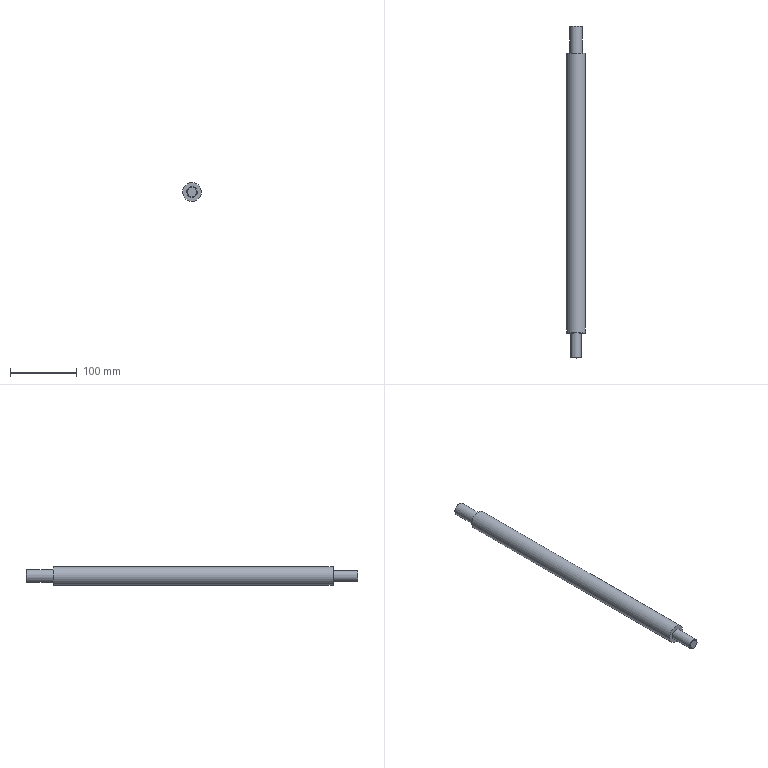Part | STEP file | SN10_003_009-03_EIXO | 1 solid | 9 faces | box 28 x 498.3 x 28 mm | volume 277666 mm3 | plane 4 | cylinder 3 | cone 2 | commonest cylinder face diameters 16 x1 19.05 x1 28 x1
STEP:
#1=CARTESIAN_POINT('',(0.,0.,0.));
#2=DIRECTION('',(0.,0.,1.));
#3=DIRECTION('',(1.,0.,0.));
#4=AXIS2_PLACEMENT_3D('',#1,#2,#3);
#5=CARTESIAN_POINT('',(993.288,42.3,12.286));
#6=VERTEX_POINT('',#5);
#7=CARTESIAN_POINT('',(1000.,42.3,0.));
#8=DIRECTION('',(0.,-1.,0.));
#9=DIRECTION('',(1.,0.,0.));
#10=AXIS2_PLACEMENT_3D('',#7,#8,#9);
#11=CIRCLE('',#10,14.);
#12=CARTESIAN_POINT('',(1000.,-165.85,0.));
#13=DIRECTION('',(0.,-1.,0.));
#14=DIRECTION('',(-0.4794,0.,0.8776));
#15=AXIS2_PLACEMENT_3D('',#12,#13,#14);
#16=CYLINDRICAL_SURFACE('',#15,14.);
#17=CARTESIAN_POINT('',(-2.071,-208.15));
#18=DIRECTION('',(1.,0.));
#19=VECTOR('',#18,1.);
#20=LINE('',#17,#19);
#21=(GEOMETRIC_REPRESENTATION_CONTEXT(2)PARAMETRIC_REPRESENTATION_CONTEXT()REPRESENTATION_CONTEXT('',''));
#22=DEFINITIONAL_REPRESENTATION('',(#20),#21);
#23=PCURVE('',#16,#22);
#24=CARTESIAN_POINT('',(1000.,42.3,14.));
#25=DIRECTION('',(0.,-1.,0.));
#26=DIRECTION('',(0.,0.,-1.));
#27=AXIS2_PLACEMENT_3D('',#24,#25,#26);
#28=PLANE('',#27);
#29=CARTESIAN_POINT('',(14.,0.));
#30=DIRECTION('',(0.,1.));
#31=AXIS2_PLACEMENT_2D('',#29,#30);
#32=CIRCLE('',#31,14.);
#33=(GEOMETRIC_REPRESENTATION_CONTEXT(2)PARAMETRIC_REPRESENTATION_CONTEXT()REPRESENTATION_CONTEXT('',''));
#34=DEFINITIONAL_REPRESENTATION('',(#32),#33);
#35=PCURVE('',#28,#34);
#36=SURFACE_CURVE('',#11,(#23,#35),.PCURVE_S1.);
#37=EDGE_CURVE('',#6,#6,#36,.T.);
#38=ORIENTED_EDGE('',*,*,#37,.T.);
#39=CARTESIAN_POINT('',(993.288,-377.5,12.286));
#40=VERTEX_POINT('',#39);
#41=CARTESIAN_POINT('',(993.288,42.3,12.286));
#42=CARTESIAN_POINT('',(993.288,-377.5,12.286));
#43=B_SPLINE_CURVE_WITH_KNOTS('',1,(#41,#42),.UNSPECIFIED.,.F.,.F.,(2,2),(-208.15,211.65),.PIECEWISE_BEZIER_KNOTS.);
#44=CARTESIAN_POINT('',(6.283,0.));
#45=DIRECTION('',(0.,1.));
#46=VECTOR('',#45,1.);
#47=LINE('',#44,#46);
#48=(GEOMETRIC_REPRESENTATION_CONTEXT(2)PARAMETRIC_REPRESENTATION_CONTEXT()REPRESENTATION_CONTEXT('',''));
#49=DEFINITIONAL_REPRESENTATION('',(#47),#48);
#50=PCURVE('',#16,#49);
#51=CARTESIAN_POINT('',(0.,0.));
#52=DIRECTION('',(0.,1.));
#53=VECTOR('',#52,1.);
#54=LINE('',#51,#53);
#55=(GEOMETRIC_REPRESENTATION_CONTEXT(2)PARAMETRIC_REPRESENTATION_CONTEXT()REPRESENTATION_CONTEXT('',''));
#56=DEFINITIONAL_REPRESENTATION('',(#54),#55);
#57=PCURVE('',#16,#56);
#58=SEAM_CURVE('',#43,(#50,#57),.PCURVE_S1.);
#59=EDGE_CURVE('',#6,#40,#58,.T.);
#60=ORIENTED_EDGE('',*,*,#59,.T.);
#61=CARTESIAN_POINT('',(1000.,-377.5,0.));
#62=DIRECTION('',(0.,-1.,0.));
#63=DIRECTION('',(1.,0.,0.));
#64=AXIS2_PLACEMENT_3D('',#61,#62,#63);
#65=CIRCLE('',#64,14.);
#66=CARTESIAN_POINT('',(-2.071,211.65));
#67=DIRECTION('',(1.,0.));
#68=VECTOR('',#67,1.);
#69=LINE('',#66,#68);
#70=(GEOMETRIC_REPRESENTATION_CONTEXT(2)PARAMETRIC_REPRESENTATION_CONTEXT()REPRESENTATION_CONTEXT('',''));
#71=DEFINITIONAL_REPRESENTATION('',(#69),#70);
#72=PCURVE('',#16,#71);
#73=CARTESIAN_POINT('',(1000.,-377.5,8.));
#74=DIRECTION('',(0.,-1.,0.));
#75=DIRECTION('',(0.,0.,-1.));
#76=AXIS2_PLACEMENT_3D('',#73,#74,#75);
#77=PLANE('',#76);
#78=CARTESIAN_POINT('',(8.,0.));
#79=DIRECTION('',(0.,1.));
#80=AXIS2_PLACEMENT_2D('',#78,#79);
#81=CIRCLE('',#80,14.);
#82=(GEOMETRIC_REPRESENTATION_CONTEXT(2)PARAMETRIC_REPRESENTATION_CONTEXT()REPRESENTATION_CONTEXT('',''));
#83=DEFINITIONAL_REPRESENTATION('',(#81),#82);
#84=PCURVE('',#77,#83);
#85=SURFACE_CURVE('',#65,(#72,#84),.PCURVE_S1.);
#86=EDGE_CURVE('',#40,#40,#85,.T.);
#87=ORIENTED_EDGE('',*,*,#86,.F.);
#88=ORIENTED_EDGE('',*,*,#59,.F.);
#89=EDGE_LOOP('',(#38,#60,#87,#88));
#90=FACE_BOUND('',#89,.T.);
#91=ADVANCED_FACE('',(#90),#16,.T.);
#92=ORIENTED_EDGE('',*,*,#37,.F.);
#93=EDGE_LOOP('',(#92));
#94=FACE_BOUND('',#93,.T.);
#95=CARTESIAN_POINT('',(995.433,42.3,8.359));
#96=VERTEX_POINT('',#95);
#97=CARTESIAN_POINT('',(1000.,42.3,0.));
#98=DIRECTION('',(0.,-1.,0.));
#99=DIRECTION('',(1.,0.,0.));
#100=AXIS2_PLACEMENT_3D('',#97,#98,#99);
#101=CIRCLE('',#100,9.525);
#102=CARTESIAN_POINT('',(14.,0.));
#103=DIRECTION('',(0.,1.));
#104=AXIS2_PLACEMENT_2D('',#102,#103);
#105=CIRCLE('',#104,9.525);
#106=(GEOMETRIC_REPRESENTATION_CONTEXT(2)PARAMETRIC_REPRESENTATION_CONTEXT()REPRESENTATION_CONTEXT('',''));
#107=DEFINITIONAL_REPRESENTATION('',(#105),#106);
#108=PCURVE('',#28,#107);
#109=CARTESIAN_POINT('',(1000.,-165.85,0.));
#110=DIRECTION('',(0.,-1.,0.));
#111=DIRECTION('',(-0.4794,0.,0.8776));
#112=AXIS2_PLACEMENT_3D('',#109,#110,#111);
#113=CYLINDRICAL_SURFACE('',#112,9.525);
#114=CARTESIAN_POINT('',(-2.071,-208.15));
#115=DIRECTION('',(1.,0.));
#116=VECTOR('',#115,1.);
#117=LINE('',#114,#116);
#118=(GEOMETRIC_REPRESENTATION_CONTEXT(2)PARAMETRIC_REPRESENTATION_CONTEXT()REPRESENTATION_CONTEXT('',''));
#119=DEFINITIONAL_REPRESENTATION('',(#117),#118);
#120=PCURVE('',#113,#119);
#121=SURFACE_CURVE('',#101,(#108,#120),.PCURVE_S1.);
#122=EDGE_CURVE('',#96,#96,#121,.T.);
#123=ORIENTED_EDGE('',*,*,#122,.T.);
#124=EDGE_LOOP('',(#123));
#125=FACE_BOUND('',#124,.T.);
#126=ADVANCED_FACE('',(#94,#125),#28,.F.);
#127=ORIENTED_EDGE('',*,*,#86,.T.);
#128=EDGE_LOOP('',(#127));
#129=FACE_BOUND('',#128,.T.);
#130=CARTESIAN_POINT('',(1003.835,-377.5,-7.021));
#131=VERTEX_POINT('',#130);
#132=CARTESIAN_POINT('',(1000.,-377.5,0.));
#133=DIRECTION('',(0.,-1.,0.));
#134=DIRECTION('',(1.,0.,0.));
#135=AXIS2_PLACEMENT_3D('',#132,#133,#134);
#136=CIRCLE('',#135,8.);
#137=CARTESIAN_POINT('',(8.,0.));
#138=DIRECTION('',(0.,1.));
#139=AXIS2_PLACEMENT_2D('',#137,#138);
#140=CIRCLE('',#139,8.);
#141=(GEOMETRIC_REPRESENTATION_CONTEXT(2)PARAMETRIC_REPRESENTATION_CONTEXT()REPRESENTATION_CONTEXT('',''));
#142=DEFINITIONAL_REPRESENTATION('',(#140),#141);
#143=PCURVE('',#77,#142);
#144=CARTESIAN_POINT('',(1000.,-165.85,0.));
#145=DIRECTION('',(0.,-1.,0.));
#146=DIRECTION('',(-0.4794,0.,0.8776));
#147=AXIS2_PLACEMENT_3D('',#144,#145,#146);
#148=CYLINDRICAL_SURFACE('',#147,8.);
#149=CARTESIAN_POINT('',(-2.071,211.65));
#150=DIRECTION('',(1.,0.));
#151=VECTOR('',#150,1.);
#152=LINE('',#149,#151);
#153=(GEOMETRIC_REPRESENTATION_CONTEXT(2)PARAMETRIC_REPRESENTATION_CONTEXT()REPRESENTATION_CONTEXT('',''));
#154=DEFINITIONAL_REPRESENTATION('',(#152),#153);
#155=PCURVE('',#148,#154);
#156=SURFACE_CURVE('',#136,(#143,#155),.PCURVE_S1.);
#157=EDGE_CURVE('',#131,#131,#156,.T.);
#158=ORIENTED_EDGE('',*,*,#157,.F.);
#159=EDGE_LOOP('',(#158));
#160=FACE_BOUND('',#159,.T.);
#161=ADVANCED_FACE('',(#129,#160),#77,.T.);
#162=CARTESIAN_POINT('',(1003.835,-414.,-7.021));
#163=VERTEX_POINT('',#162);
#164=CARTESIAN_POINT('',(1000.,-414.,0.));
#165=DIRECTION('',(0.,-1.,0.));
#166=DIRECTION('',(1.,0.,0.));
#167=AXIS2_PLACEMENT_3D('',#164,#165,#166);
#168=CIRCLE('',#167,8.);
#169=CARTESIAN_POINT('',(-2.071,248.15));
#170=DIRECTION('',(1.,0.));
#171=VECTOR('',#170,1.);
#172=LINE('',#169,#171);
#173=(GEOMETRIC_REPRESENTATION_CONTEXT(2)PARAMETRIC_REPRESENTATION_CONTEXT()REPRESENTATION_CONTEXT('',''));
#174=DEFINITIONAL_REPRESENTATION('',(#172),#173);
#175=PCURVE('',#148,#174);
#176=CARTESIAN_POINT('',(1000.,-421.,0.));
#177=DIRECTION('',(0.,1.,0.));
#178=DIRECTION('',(0.1376,0.,-0.9905));
#179=AXIS2_PLACEMENT_3D('',#176,#177,#178);
#180=CONICAL_SURFACE('',#179,1.,0.7854);
#181=CARTESIAN_POINT('',(17.417,7.));
#182=DIRECTION('',(-1.,0.));
#183=VECTOR('',#182,1.);
#184=LINE('',#181,#183);
#185=(GEOMETRIC_REPRESENTATION_CONTEXT(2)PARAMETRIC_REPRESENTATION_CONTEXT()REPRESENTATION_CONTEXT('',''));
#186=DEFINITIONAL_REPRESENTATION('',(#184),#185);
#187=PCURVE('',#180,#186);
#188=SURFACE_CURVE('',#168,(#175,#187),.PCURVE_S1.);
#189=EDGE_CURVE('',#163,#163,#188,.T.);
#190=ORIENTED_EDGE('',*,*,#189,.F.);
#191=CARTESIAN_POINT('',(1003.835,-377.5,-7.021));
#192=CARTESIAN_POINT('',(1003.835,-414.,-7.021));
#193=B_SPLINE_CURVE_WITH_KNOTS('',1,(#191,#192),.UNSPECIFIED.,.F.,.F.,(2,2),(211.65,248.15),.PIECEWISE_BEZIER_KNOTS.);
#194=CARTESIAN_POINT('',(3.142,0.));
#195=DIRECTION('',(0.,1.));
#196=VECTOR('',#195,1.);
#197=LINE('',#194,#196);
#198=(GEOMETRIC_REPRESENTATION_CONTEXT(2)PARAMETRIC_REPRESENTATION_CONTEXT()REPRESENTATION_CONTEXT('',''));
#199=DEFINITIONAL_REPRESENTATION('',(#197),#198);
#200=PCURVE('',#148,#199);
#201=CARTESIAN_POINT('',(9.425,0.));
#202=DIRECTION('',(0.,1.));
#203=VECTOR('',#202,1.);
#204=LINE('',#201,#203);
#205=(GEOMETRIC_REPRESENTATION_CONTEXT(2)PARAMETRIC_REPRESENTATION_CONTEXT()REPRESENTATION_CONTEXT('',''));
#206=DEFINITIONAL_REPRESENTATION('',(#204),#205);
#207=PCURVE('',#148,#206);
#208=SEAM_CURVE('',#193,(#200,#207),.PCURVE_S1.);
#209=EDGE_CURVE('',#131,#163,#208,.T.);
#210=ORIENTED_EDGE('',*,*,#209,.F.);
#211=ORIENTED_EDGE('',*,*,#157,.T.);
#212=ORIENTED_EDGE('',*,*,#209,.T.);
#213=EDGE_LOOP('',(#190,#210,#211,#212));
#214=FACE_BOUND('',#213,.T.);
#215=ADVANCED_FACE('',(#214),#148,.T.);
#216=CARTESIAN_POINT('',(996.644,-415.,6.143));
#217=VERTEX_POINT('',#216);
#218=CARTESIAN_POINT('',(1003.356,-415.,-6.143));
#219=VERTEX_POINT('',#218);
#220=CARTESIAN_POINT('',(1000.,-415.,0.));
#221=DIRECTION('',(0.,-1.,0.));
#222=DIRECTION('',(1.,0.,0.));
#223=AXIS2_PLACEMENT_3D('',#220,#221,#222);
#224=CIRCLE('',#223,7.);
#225=CARTESIAN_POINT('',(1000.,-415.,0.));
#226=DIRECTION('',(0.,-1.,0.));
#227=DIRECTION('',(0.,0.,-1.));
#228=AXIS2_PLACEMENT_3D('',#225,#226,#227);
#229=PLANE('',#228);
#230=CARTESIAN_POINT('',(0.,0.));
#231=DIRECTION('',(0.,1.));
#232=AXIS2_PLACEMENT_2D('',#230,#231);
#233=CIRCLE('',#232,7.);
#234=(GEOMETRIC_REPRESENTATION_CONTEXT(2)PARAMETRIC_REPRESENTATION_CONTEXT()REPRESENTATION_CONTEXT('',''));
#235=DEFINITIONAL_REPRESENTATION('',(#233),#234);
#236=PCURVE('',#229,#235);
#237=CARTESIAN_POINT('',(11.134,6.));
#238=DIRECTION('',(-1.,0.));
#239=VECTOR('',#238,1.);
#240=LINE('',#237,#239);
#241=(GEOMETRIC_REPRESENTATION_CONTEXT(2)PARAMETRIC_REPRESENTATION_CONTEXT()REPRESENTATION_CONTEXT('',''));
#242=DEFINITIONAL_REPRESENTATION('',(#240),#241);
#243=PCURVE('',#180,#242);
#244=SURFACE_CURVE('',#224,(#236,#243),.PCURVE_S1.);
#245=EDGE_CURVE('',#217,#219,#244,.T.);
#246=ORIENTED_EDGE('',*,*,#245,.T.);
#247=CARTESIAN_POINT('',(1000.,-415.,0.));
#248=DIRECTION('',(0.,-1.,0.));
#249=DIRECTION('',(1.,0.,0.));
#250=AXIS2_PLACEMENT_3D('',#247,#248,#249);
#251=CIRCLE('',#250,7.);
#252=CARTESIAN_POINT('',(0.,0.));
#253=DIRECTION('',(0.,1.));
#254=AXIS2_PLACEMENT_2D('',#252,#253);
#255=CIRCLE('',#254,7.);
#256=(GEOMETRIC_REPRESENTATION_CONTEXT(2)PARAMETRIC_REPRESENTATION_CONTEXT()REPRESENTATION_CONTEXT('',''));
#257=DEFINITIONAL_REPRESENTATION('',(#255),#256);
#258=PCURVE('',#229,#257);
#259=CARTESIAN_POINT('',(17.417,6.));
#260=DIRECTION('',(-1.,0.));
#261=VECTOR('',#260,1.);
#262=LINE('',#259,#261);
#263=(GEOMETRIC_REPRESENTATION_CONTEXT(2)PARAMETRIC_REPRESENTATION_CONTEXT()REPRESENTATION_CONTEXT('',''));
#264=DEFINITIONAL_REPRESENTATION('',(#262),#263);
#265=PCURVE('',#180,#264);
#266=SURFACE_CURVE('',#251,(#258,#265),.PCURVE_S1.);
#267=EDGE_CURVE('',#219,#217,#266,.T.);
#268=ORIENTED_EDGE('',*,*,#267,.T.);
#269=EDGE_LOOP('',(#246,#268));
#270=FACE_BOUND('',#269,.T.);
#271=ADVANCED_FACE('',(#270),#229,.T.);
#272=ORIENTED_EDGE('',*,*,#267,.F.);
#273=CARTESIAN_POINT('',(1003.356,-415.,-6.143));
#274=CARTESIAN_POINT('',(1003.835,-414.,-7.021));
#275=B_SPLINE_CURVE_WITH_KNOTS('',1,(#273,#274),.UNSPECIFIED.,.F.,.F.,(2,2),(8.485,9.899),.PIECEWISE_BEZIER_KNOTS.);
#276=CARTESIAN_POINT('',(12.204,0.));
#277=DIRECTION('',(0.,1.));
#278=VECTOR('',#277,1.);
#279=LINE('',#276,#278);
#280=(GEOMETRIC_REPRESENTATION_CONTEXT(2)PARAMETRIC_REPRESENTATION_CONTEXT()REPRESENTATION_CONTEXT('',''));
#281=DEFINITIONAL_REPRESENTATION('',(#279),#280);
#282=PCURVE('',#180,#281);
#283=CARTESIAN_POINT('',(5.921,0.));
#284=DIRECTION('',(0.,1.));
#285=VECTOR('',#284,1.);
#286=LINE('',#283,#285);
#287=(GEOMETRIC_REPRESENTATION_CONTEXT(2)PARAMETRIC_REPRESENTATION_CONTEXT()REPRESENTATION_CONTEXT('',''));
#288=DEFINITIONAL_REPRESENTATION('',(#286),#287);
#289=PCURVE('',#180,#288);
#290=SEAM_CURVE('',#275,(#282,#289),.PCURVE_S1.);
#291=EDGE_CURVE('',#219,#163,#290,.T.);
#292=ORIENTED_EDGE('',*,*,#291,.T.);
#293=ORIENTED_EDGE('',*,*,#189,.T.);
#294=ORIENTED_EDGE('',*,*,#291,.F.);
#295=ORIENTED_EDGE('',*,*,#245,.F.);
#296=EDGE_LOOP('',(#272,#292,#293,#294,#295));
#297=FACE_BOUND('',#296,.T.);
#298=ADVANCED_FACE('',(#297),#180,.T.);
#299=CARTESIAN_POINT('',(995.433,82.3,8.359));
#300=VERTEX_POINT('',#299);
#301=CARTESIAN_POINT('',(1000.,82.3,0.));
#302=DIRECTION('',(0.,-1.,0.));
#303=DIRECTION('',(1.,0.,0.));
#304=AXIS2_PLACEMENT_3D('',#301,#302,#303);
#305=CIRCLE('',#304,9.525);
#306=CARTESIAN_POINT('',(-2.071,-248.15));
#307=DIRECTION('',(1.,0.));
#308=VECTOR('',#307,1.);
#309=LINE('',#306,#308);
#310=(GEOMETRIC_REPRESENTATION_CONTEXT(2)PARAMETRIC_REPRESENTATION_CONTEXT()REPRESENTATION_CONTEXT('',''));
#311=DEFINITIONAL_REPRESENTATION('',(#309),#310);
#312=PCURVE('',#113,#311);
#313=CARTESIAN_POINT('',(1000.,90.825,0.));
#314=DIRECTION('',(0.,-1.,0.));
#315=DIRECTION('',(0.4621,0.,-0.8868));
#316=AXIS2_PLACEMENT_3D('',#313,#314,#315);
#317=CONICAL_SURFACE('',#316,1.,0.7854);
#318=CARTESIAN_POINT('',(1.09,8.525));
#319=DIRECTION('',(1.,0.));
#320=VECTOR('',#319,1.);
#321=LINE('',#318,#320);
#322=(GEOMETRIC_REPRESENTATION_CONTEXT(2)PARAMETRIC_REPRESENTATION_CONTEXT()REPRESENTATION_CONTEXT('',''));
#323=DEFINITIONAL_REPRESENTATION('',(#321),#322);
#324=PCURVE('',#317,#323);
#325=SURFACE_CURVE('',#305,(#312,#324),.PCURVE_S1.);
#326=EDGE_CURVE('',#300,#300,#325,.T.);
#327=ORIENTED_EDGE('',*,*,#326,.T.);
#328=CARTESIAN_POINT('',(995.433,82.3,8.359));
#329=CARTESIAN_POINT('',(995.433,42.3,8.359));
#330=B_SPLINE_CURVE_WITH_KNOTS('',1,(#328,#329),.UNSPECIFIED.,.F.,.F.,(2,2),(-248.15,-208.15),.PIECEWISE_BEZIER_KNOTS.);
#331=CARTESIAN_POINT('',(6.283,0.));
#332=DIRECTION('',(0.,1.));
#333=VECTOR('',#332,1.);
#334=LINE('',#331,#333);
#335=(GEOMETRIC_REPRESENTATION_CONTEXT(2)PARAMETRIC_REPRESENTATION_CONTEXT()REPRESENTATION_CONTEXT('',''));
#336=DEFINITIONAL_REPRESENTATION('',(#334),#335);
#337=PCURVE('',#113,#336);
#338=CARTESIAN_POINT('',(0.,0.));
#339=DIRECTION('',(0.,1.));
#340=VECTOR('',#339,1.);
#341=LINE('',#338,#340);
#342=(GEOMETRIC_REPRESENTATION_CONTEXT(2)PARAMETRIC_REPRESENTATION_CONTEXT()REPRESENTATION_CONTEXT('',''));
#343=DEFINITIONAL_REPRESENTATION('',(#341),#342);
#344=PCURVE('',#113,#343);
#345=SEAM_CURVE('',#330,(#337,#344),.PCURVE_S1.);
#346=EDGE_CURVE('',#300,#96,#345,.T.);
#347=ORIENTED_EDGE('',*,*,#346,.T.);
#348=ORIENTED_EDGE('',*,*,#122,.F.);
#349=ORIENTED_EDGE('',*,*,#346,.F.);
#350=EDGE_LOOP('',(#327,#347,#348,#349));
#351=FACE_BOUND('',#350,.T.);
#352=ADVANCED_FACE('',(#351),#113,.T.);
#353=CARTESIAN_POINT('',(995.913,83.3,7.481));
#354=VERTEX_POINT('',#353);
#355=CARTESIAN_POINT('',(1000.,83.3,0.));
#356=DIRECTION('',(0.,-1.,0.));
#357=DIRECTION('',(1.,0.,0.));
#358=AXIS2_PLACEMENT_3D('',#355,#356,#357);
#359=CIRCLE('',#358,8.525);
#360=CARTESIAN_POINT('',(1000.,83.3,9.525));
#361=DIRECTION('',(0.,-1.,0.));
#362=DIRECTION('',(0.,0.,-1.));
#363=AXIS2_PLACEMENT_3D('',#360,#361,#362);
#364=PLANE('',#363);
#365=CARTESIAN_POINT('',(9.525,0.));
#366=DIRECTION('',(0.,1.));
#367=AXIS2_PLACEMENT_2D('',#365,#366);
#368=CIRCLE('',#367,8.525);
#369=(GEOMETRIC_REPRESENTATION_CONTEXT(2)PARAMETRIC_REPRESENTATION_CONTEXT()REPRESENTATION_CONTEXT('',''));
#370=DEFINITIONAL_REPRESENTATION('',(#368),#369);
#371=PCURVE('',#364,#370);
#372=CARTESIAN_POINT('',(1.09,7.525));
#373=DIRECTION('',(1.,0.));
#374=VECTOR('',#373,1.);
#375=LINE('',#372,#374);
#376=(GEOMETRIC_REPRESENTATION_CONTEXT(2)PARAMETRIC_REPRESENTATION_CONTEXT()REPRESENTATION_CONTEXT('',''));
#377=DEFINITIONAL_REPRESENTATION('',(#375),#376);
#378=PCURVE('',#317,#377);
#379=SURFACE_CURVE('',#359,(#371,#378),.PCURVE_S1.);
#380=EDGE_CURVE('',#354,#354,#379,.T.);
#381=ORIENTED_EDGE('',*,*,#380,.F.);
#382=EDGE_LOOP('',(#381));
#383=FACE_BOUND('',#382,.T.);
#384=ADVANCED_FACE('',(#383),#364,.F.);
#385=ORIENTED_EDGE('',*,*,#326,.F.);
#386=CARTESIAN_POINT('',(995.913,83.3,7.481));
#387=CARTESIAN_POINT('',(995.433,82.3,8.359));
#388=B_SPLINE_CURVE_WITH_KNOTS('',1,(#386,#387),.UNSPECIFIED.,.F.,.F.,(2,2),(10.642,12.056),.PIECEWISE_BEZIER_KNOTS.);
#389=CARTESIAN_POINT('',(3.161,0.));
#390=DIRECTION('',(0.,1.));
#391=VECTOR('',#390,1.);
#392=LINE('',#389,#391);
#393=(GEOMETRIC_REPRESENTATION_CONTEXT(2)PARAMETRIC_REPRESENTATION_CONTEXT()REPRESENTATION_CONTEXT('',''));
#394=DEFINITIONAL_REPRESENTATION('',(#392),#393);
#395=PCURVE('',#317,#394);
#396=CARTESIAN_POINT('',(9.444,0.));
#397=DIRECTION('',(0.,1.));
#398=VECTOR('',#397,1.);
#399=LINE('',#396,#398);
#400=(GEOMETRIC_REPRESENTATION_CONTEXT(2)PARAMETRIC_REPRESENTATION_CONTEXT()REPRESENTATION_CONTEXT('',''));
#401=DEFINITIONAL_REPRESENTATION('',(#399),#400);
#402=PCURVE('',#317,#401);
#403=SEAM_CURVE('',#388,(#395,#402),.PCURVE_S1.);
#404=EDGE_CURVE('',#354,#300,#403,.T.);
#405=ORIENTED_EDGE('',*,*,#404,.F.);
#406=ORIENTED_EDGE('',*,*,#380,.T.);
#407=ORIENTED_EDGE('',*,*,#404,.T.);
#408=EDGE_LOOP('',(#385,#405,#406,#407));
#409=FACE_BOUND('',#408,.T.);
#410=ADVANCED_FACE('',(#409),#317,.T.);
#411=CLOSED_SHELL('',(#91,#126,#161,#215,#271,#298,#352,#384,#410));
#412=MANIFOLD_SOLID_BREP('',#411);
#413=(LENGTH_UNIT()NAMED_UNIT(*)SI_UNIT(.MILLI.,.METRE.));
#414=UNCERTAINTY_MEASURE_WITH_UNIT(LENGTH_MEASURE(0.00001),#413,'','');
#415=(NAMED_UNIT(*)PLANE_ANGLE_UNIT()SI_UNIT($,.RADIAN.));
#416=(NAMED_UNIT(*)SI_UNIT($,.STERADIAN.)SOLID_ANGLE_UNIT());
#417=(GEOMETRIC_REPRESENTATION_CONTEXT(3)GLOBAL_UNCERTAINTY_ASSIGNED_CONTEXT((#414))GLOBAL_UNIT_ASSIGNED_CONTEXT((#413,#415,#416))REPRESENTATION_CONTEXT('',''));
#418=ADVANCED_BREP_SHAPE_REPRESENTATION('',(#4,#412),#417);